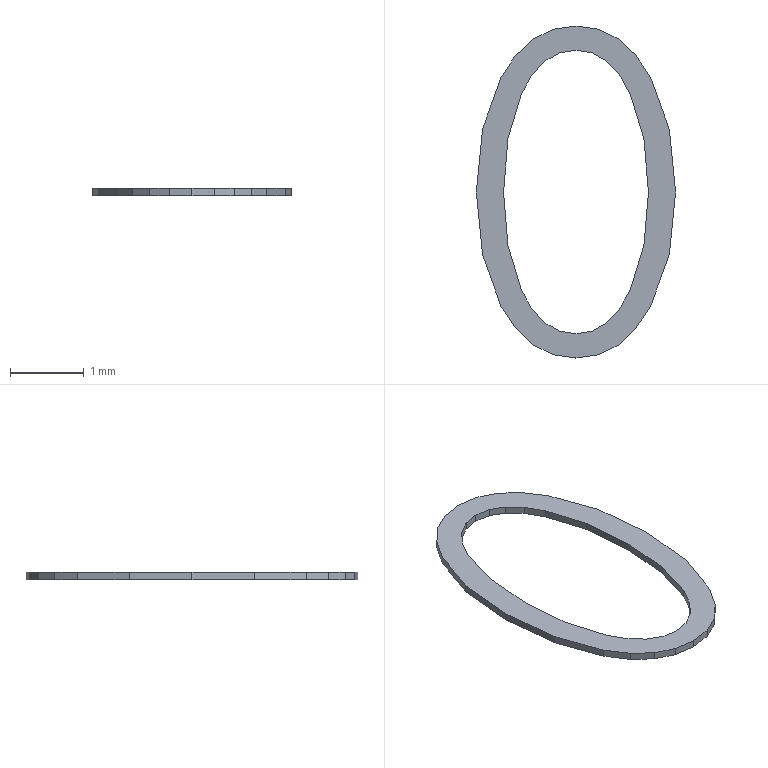Part | STEP file | PART243.stp | 1 solid | 50 faces | box 2.692 x 4.487 x 0.1 mm | volume 0.3611 mm3 | plane 50